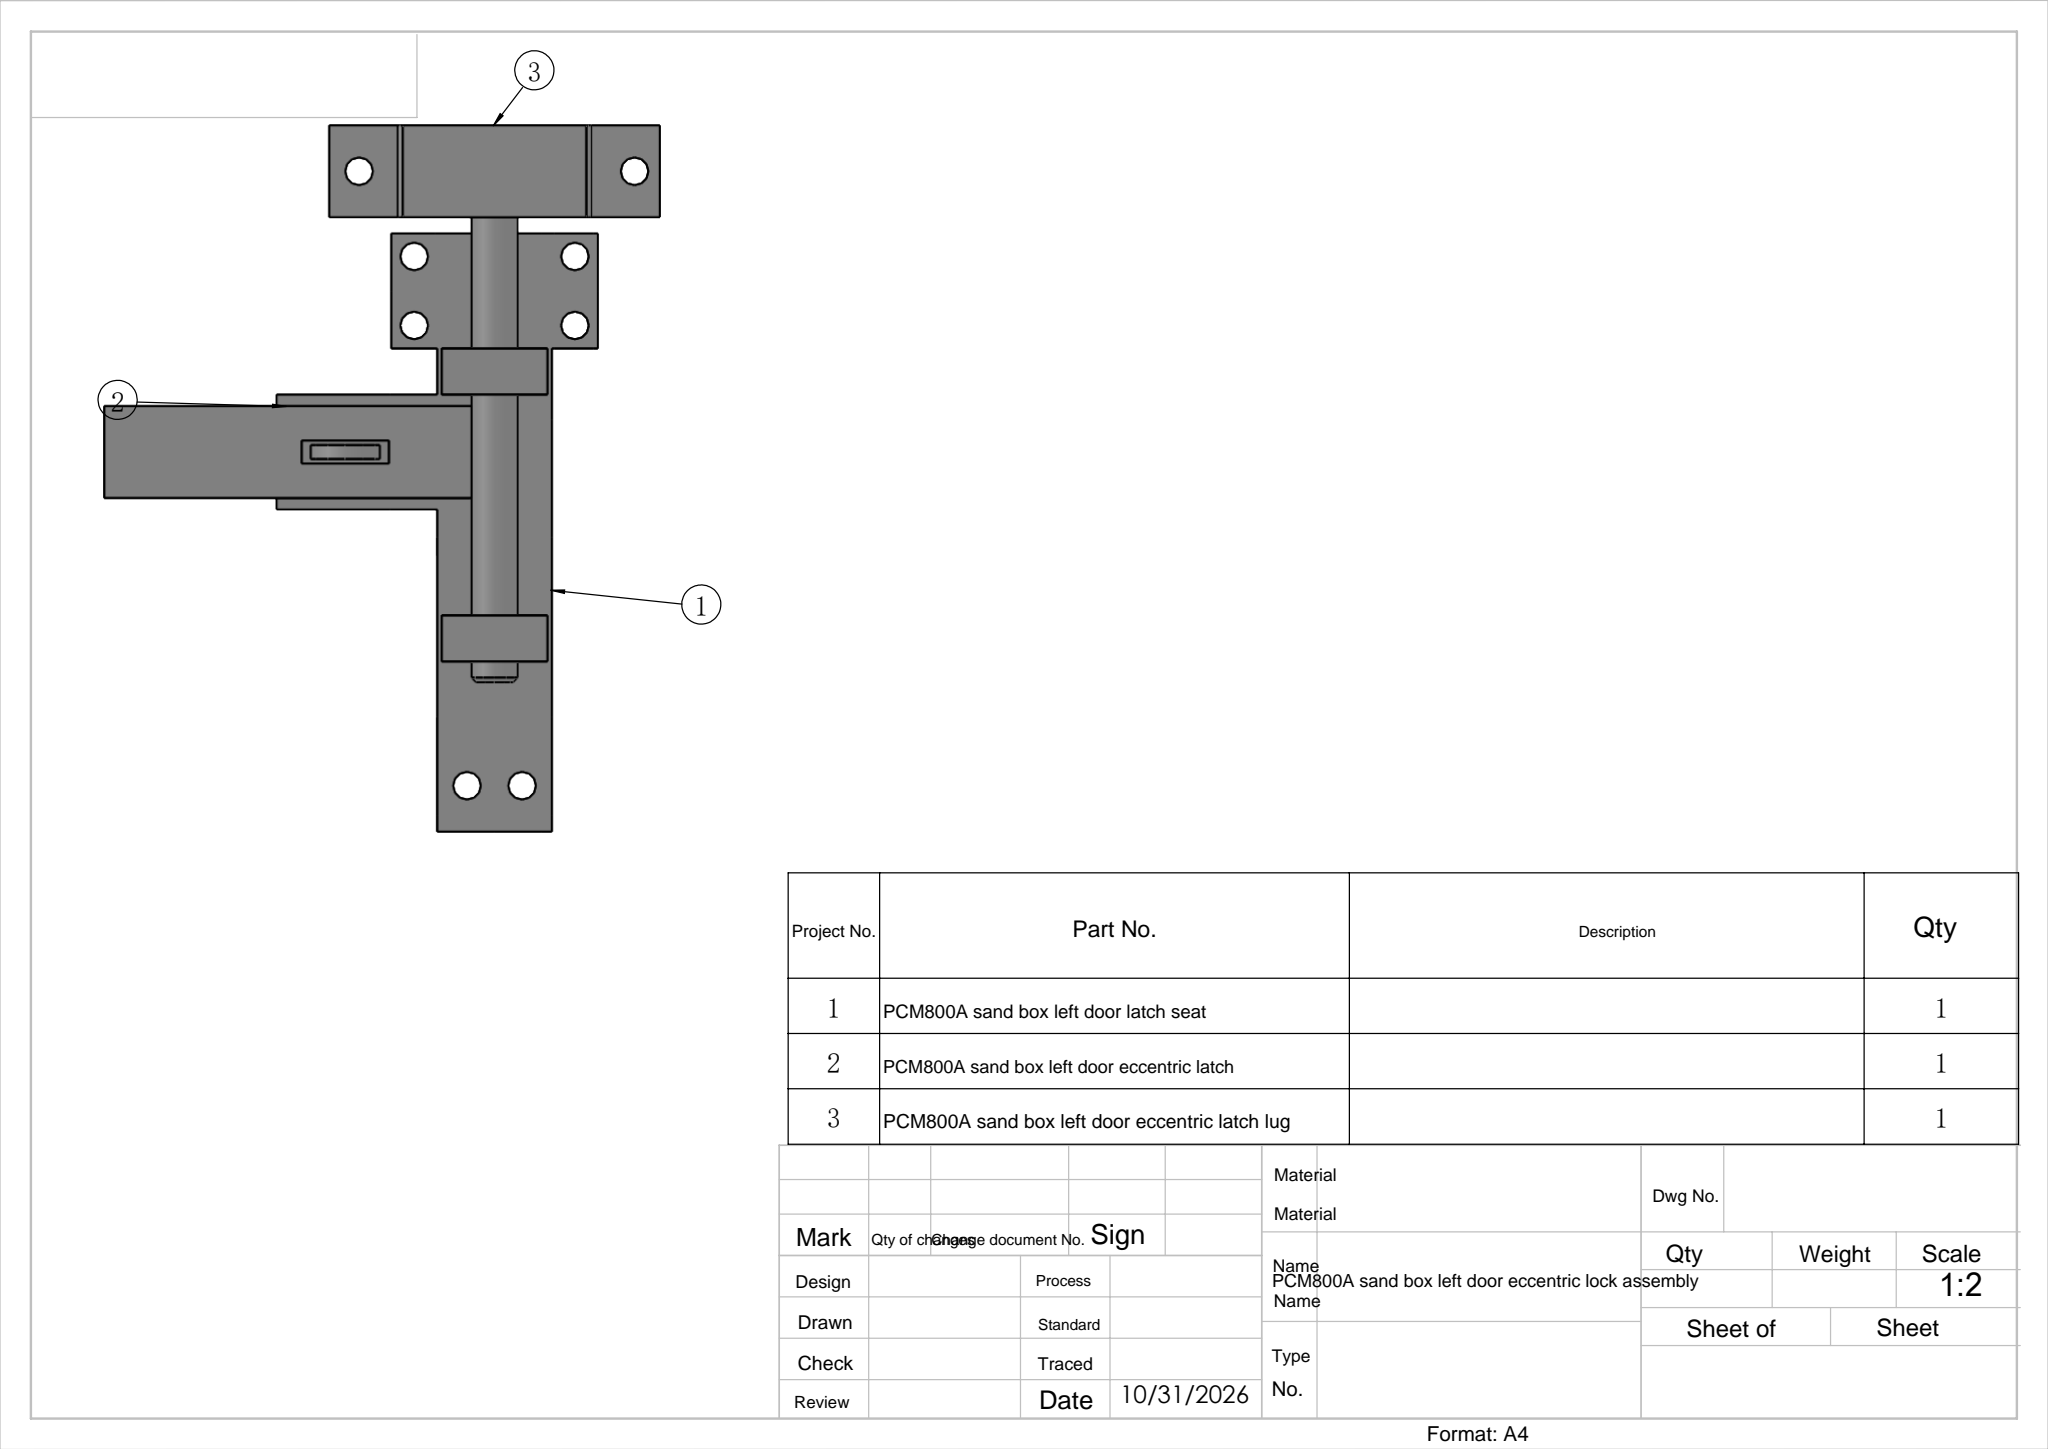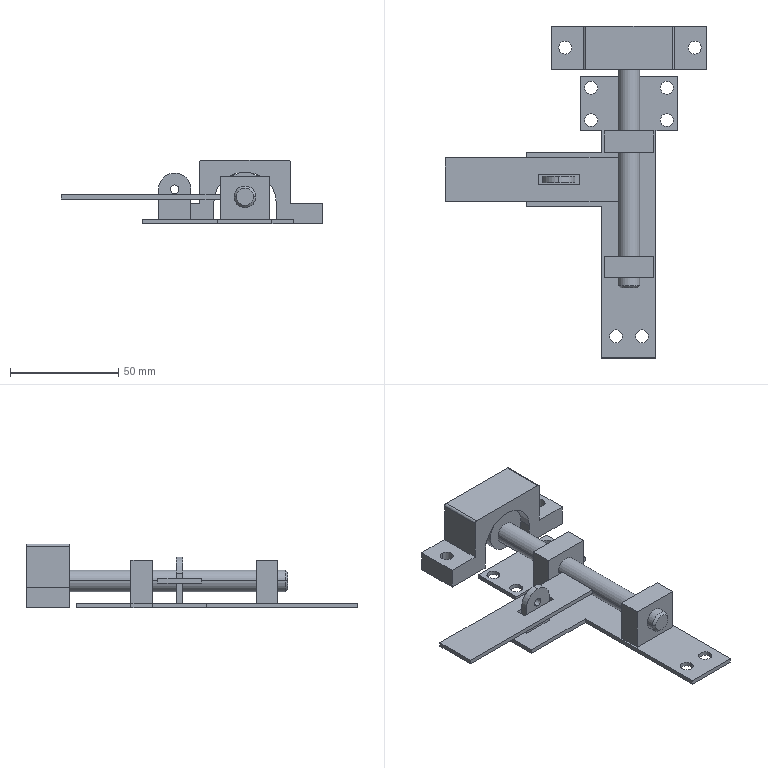Part | SolidWorks | 4 solids | 92 faces | box 121 x 153.5 x 29.5 mm | volume 51392 mm3 | plane 55 | cylinder 33 | cone 4 | commonest cylinder face diameters 6 x16 10 x8 2 x2 4 x2 15 x2 20 x2